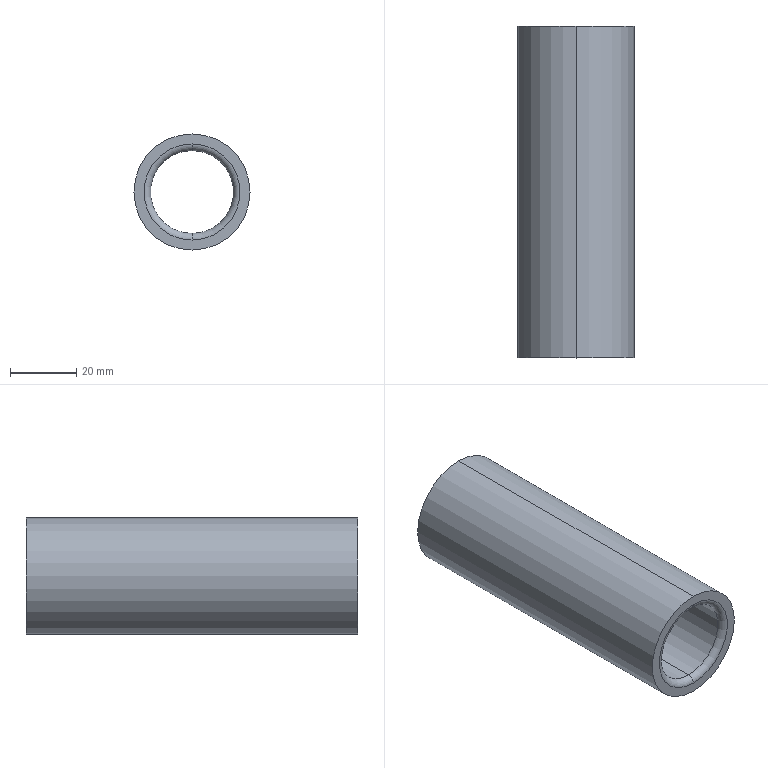Part | SolidWorks | features Extrusion 1, Fillet 1 | 1 solid | 8 faces | box 35 x 100 x 35 mm | volume 47054 mm3 | cylinder 4 | torus 2 | plane 2 | commonest cylinder face diameters 25 x2 35 x2
STEP:
#1=CARTESIAN_POINT('',(0.,2.,-12.5));
#2=VERTEX_POINT('',#1);
#3=CARTESIAN_POINT('',(0.,2.,12.5));
#4=VERTEX_POINT('',#3);
#5=CARTESIAN_POINT('',(0.,2.,0.));
#6=DIRECTION('',(0.,-1.,0.));
#7=DIRECTION('',(0.,0.,1.));
#8=AXIS2_PLACEMENT_3D('',#5,#6,#7);
#9=CIRCLE('',#8,12.5);
#10=EDGE_CURVE('',#2,#4,#9,.T.);
#11=ORIENTED_EDGE('',*,*,#10,.F.);
#12=CARTESIAN_POINT('',(0.,0.,-14.5));
#13=VERTEX_POINT('',#12);
#14=CARTESIAN_POINT('',(0.,2.,-14.5));
#15=DIRECTION('',(1.,0.,0.));
#16=DIRECTION('',(0.,0.,-1.));
#17=AXIS2_PLACEMENT_3D('',#14,#15,#16);
#18=CIRCLE('',#17,2.);
#19=EDGE_CURVE('',#2,#13,#18,.T.);
#20=ORIENTED_EDGE('',*,*,#19,.T.);
#21=CARTESIAN_POINT('',(0.,0.,14.5));
#22=VERTEX_POINT('',#21);
#23=CARTESIAN_POINT('',(0.,0.,0.));
#24=DIRECTION('',(0.,1.,0.));
#25=DIRECTION('',(0.,0.,1.));
#26=AXIS2_PLACEMENT_3D('',#23,#24,#25);
#27=CIRCLE('',#26,14.5);
#28=EDGE_CURVE('',#22,#13,#27,.T.);
#29=ORIENTED_EDGE('',*,*,#28,.F.);
#30=CARTESIAN_POINT('',(0.,2.,14.5));
#31=DIRECTION('',(-1.,0.,0.));
#32=DIRECTION('',(0.,0.,1.));
#33=AXIS2_PLACEMENT_3D('',#30,#31,#32);
#34=CIRCLE('',#33,2.);
#35=EDGE_CURVE('',#4,#22,#34,.T.);
#36=ORIENTED_EDGE('',*,*,#35,.F.);
#37=EDGE_LOOP('',(#11,#20,#29,#36));
#38=FACE_OUTER_BOUND('',#37,.T.);
#39=CARTESIAN_POINT('',(0.,2.,0.));
#40=DIRECTION('',(0.,1.,0.));
#41=DIRECTION('',(0.,0.,1.));
#42=AXIS2_PLACEMENT_3D('',#39,#40,#41);
#43=TOROIDAL_SURFACE('',#42,14.5,2.);
#44=ADVANCED_FACE('',(#38),#43,.T.);
#45=CARTESIAN_POINT('',(0.,100.,-12.5));
#46=VERTEX_POINT('',#45);
#47=CARTESIAN_POINT('',(0.,100.,12.5));
#48=VERTEX_POINT('',#47);
#49=CARTESIAN_POINT('',(0.,100.,0.));
#50=DIRECTION('',(0.,1.,0.));
#51=DIRECTION('',(0.,0.,1.));
#52=AXIS2_PLACEMENT_3D('',#49,#50,#51);
#53=CIRCLE('',#52,12.5);
#54=EDGE_CURVE('',#46,#48,#53,.T.);
#55=ORIENTED_EDGE('',*,*,#54,.T.);
#56=CARTESIAN_POINT('',(0.,100.,12.5));
#57=DIRECTION('',(0.,-1.,0.));
#58=VECTOR('',#57,1000.);
#59=LINE('',#56,#58);
#60=EDGE_CURVE('',#48,#4,#59,.T.);
#61=ORIENTED_EDGE('',*,*,#60,.T.);
#62=CARTESIAN_POINT('',(0.,2.,0.));
#63=DIRECTION('',(0.,-1.,0.));
#64=DIRECTION('',(0.,0.,1.));
#65=AXIS2_PLACEMENT_3D('',#62,#63,#64);
#66=CIRCLE('',#65,12.5);
#67=EDGE_CURVE('',#4,#2,#66,.T.);
#68=ORIENTED_EDGE('',*,*,#67,.T.);
#69=CARTESIAN_POINT('',(0.,100.,-12.5));
#70=DIRECTION('',(0.,-1.,0.));
#71=VECTOR('',#70,1000.);
#72=LINE('',#69,#71);
#73=EDGE_CURVE('',#46,#2,#72,.T.);
#74=ORIENTED_EDGE('',*,*,#73,.F.);
#75=EDGE_LOOP('',(#55,#61,#68,#74));
#76=FACE_OUTER_BOUND('',#75,.T.);
#77=CARTESIAN_POINT('',(0.,100.,0.));
#78=DIRECTION('',(0.,-1.,0.));
#79=DIRECTION('',(0.,0.,-1.));
#80=AXIS2_PLACEMENT_3D('',#77,#78,#79);
#81=CYLINDRICAL_SURFACE('',#80,12.5);
#82=ADVANCED_FACE('',(#76),#81,.F.);
#83=CARTESIAN_POINT('',(0.,100.,17.5));
#84=VERTEX_POINT('',#83);
#85=CARTESIAN_POINT('',(0.,100.,-17.5));
#86=VERTEX_POINT('',#85);
#87=CARTESIAN_POINT('',(0.,100.,0.));
#88=DIRECTION('',(0.,1.,0.));
#89=DIRECTION('',(0.,0.,1.));
#90=AXIS2_PLACEMENT_3D('',#87,#88,#89);
#91=CIRCLE('',#90,17.5);
#92=EDGE_CURVE('',#84,#86,#91,.T.);
#93=ORIENTED_EDGE('',*,*,#92,.F.);
#94=CARTESIAN_POINT('',(0.,0.,17.5));
#95=VERTEX_POINT('',#94);
#96=CARTESIAN_POINT('',(0.,100.,17.5));
#97=DIRECTION('',(0.,-1.,0.));
#98=VECTOR('',#97,1000.);
#99=LINE('',#96,#98);
#100=EDGE_CURVE('',#84,#95,#99,.T.);
#101=ORIENTED_EDGE('',*,*,#100,.T.);
#102=CARTESIAN_POINT('',(0.,0.,-17.5));
#103=VERTEX_POINT('',#102);
#104=CARTESIAN_POINT('',(0.,0.,0.));
#105=DIRECTION('',(0.,1.,0.));
#106=DIRECTION('',(0.,0.,1.));
#107=AXIS2_PLACEMENT_3D('',#104,#105,#106);
#108=CIRCLE('',#107,17.5);
#109=EDGE_CURVE('',#95,#103,#108,.T.);
#110=ORIENTED_EDGE('',*,*,#109,.T.);
#111=CARTESIAN_POINT('',(0.,100.,-17.5));
#112=DIRECTION('',(0.,-1.,0.));
#113=VECTOR('',#112,1000.);
#114=LINE('',#111,#113);
#115=EDGE_CURVE('',#86,#103,#114,.T.);
#116=ORIENTED_EDGE('',*,*,#115,.F.);
#117=EDGE_LOOP('',(#93,#101,#110,#116));
#118=FACE_OUTER_BOUND('',#117,.T.);
#119=CARTESIAN_POINT('',(0.,100.,0.));
#120=DIRECTION('',(0.,-1.,0.));
#121=DIRECTION('',(0.,0.,-1.));
#122=AXIS2_PLACEMENT_3D('',#119,#120,#121);
#123=CYLINDRICAL_SURFACE('',#122,17.5);
#124=ADVANCED_FACE('',(#118),#123,.T.);
#125=CARTESIAN_POINT('',(0.,100.,0.));
#126=DIRECTION('',(0.,1.,0.));
#127=DIRECTION('',(0.,0.,1.));
#128=AXIS2_PLACEMENT_3D('',#125,#126,#127);
#129=CIRCLE('',#128,17.5);
#130=EDGE_CURVE('',#86,#84,#129,.T.);
#131=ORIENTED_EDGE('',*,*,#130,.T.);
#132=ORIENTED_EDGE('',*,*,#92,.T.);
#133=EDGE_LOOP('',(#131,#132));
#134=FACE_OUTER_BOUND('',#133,.T.);
#135=ORIENTED_EDGE('',*,*,#54,.F.);
#136=CARTESIAN_POINT('',(0.,100.,0.));
#137=DIRECTION('',(0.,1.,0.));
#138=DIRECTION('',(0.,0.,1.));
#139=AXIS2_PLACEMENT_3D('',#136,#137,#138);
#140=CIRCLE('',#139,12.5);
#141=EDGE_CURVE('',#48,#46,#140,.T.);
#142=ORIENTED_EDGE('',*,*,#141,.F.);
#143=EDGE_LOOP('',(#135,#142));
#144=FACE_BOUND('',#143,.T.);
#145=CARTESIAN_POINT('',(0.,100.,0.));
#146=DIRECTION('',(0.,1.,0.));
#147=DIRECTION('',(0.,0.,1.));
#148=AXIS2_PLACEMENT_3D('',#145,#146,#147);
#149=PLANE('',#148);
#150=ADVANCED_FACE('',(#134,#144),#149,.T.);
#151=ORIENTED_EDGE('',*,*,#28,.T.);
#152=CARTESIAN_POINT('',(0.,0.,0.));
#153=DIRECTION('',(0.,1.,0.));
#154=DIRECTION('',(0.,0.,1.));
#155=AXIS2_PLACEMENT_3D('',#152,#153,#154);
#156=CIRCLE('',#155,14.5);
#157=EDGE_CURVE('',#13,#22,#156,.T.);
#158=ORIENTED_EDGE('',*,*,#157,.T.);
#159=EDGE_LOOP('',(#151,#158));
#160=FACE_BOUND('',#159,.T.);
#161=CARTESIAN_POINT('',(0.,0.,0.));
#162=DIRECTION('',(0.,1.,0.));
#163=DIRECTION('',(0.,0.,1.));
#164=AXIS2_PLACEMENT_3D('',#161,#162,#163);
#165=CIRCLE('',#164,17.5);
#166=EDGE_CURVE('',#103,#95,#165,.T.);
#167=ORIENTED_EDGE('',*,*,#166,.F.);
#168=ORIENTED_EDGE('',*,*,#109,.F.);
#169=EDGE_LOOP('',(#167,#168));
#170=FACE_OUTER_BOUND('',#169,.T.);
#171=CARTESIAN_POINT('',(0.,0.,0.));
#172=DIRECTION('',(0.,1.,0.));
#173=DIRECTION('',(0.,0.,1.));
#174=AXIS2_PLACEMENT_3D('',#171,#172,#173);
#175=PLANE('',#174);
#176=ADVANCED_FACE('',(#160,#170),#175,.F.);
#177=ORIENTED_EDGE('',*,*,#100,.F.);
#178=ORIENTED_EDGE('',*,*,#130,.F.);
#179=ORIENTED_EDGE('',*,*,#115,.T.);
#180=ORIENTED_EDGE('',*,*,#166,.T.);
#181=EDGE_LOOP('',(#177,#178,#179,#180));
#182=FACE_OUTER_BOUND('',#181,.T.);
#183=CARTESIAN_POINT('',(0.,100.,0.));
#184=DIRECTION('',(0.,-1.,0.));
#185=DIRECTION('',(0.,0.,-1.));
#186=AXIS2_PLACEMENT_3D('',#183,#184,#185);
#187=CYLINDRICAL_SURFACE('',#186,17.5);
#188=ADVANCED_FACE('',(#182),#187,.T.);
#189=ORIENTED_EDGE('',*,*,#60,.F.);
#190=ORIENTED_EDGE('',*,*,#141,.T.);
#191=ORIENTED_EDGE('',*,*,#73,.T.);
#192=ORIENTED_EDGE('',*,*,#10,.T.);
#193=EDGE_LOOP('',(#189,#190,#191,#192));
#194=FACE_OUTER_BOUND('',#193,.T.);
#195=CARTESIAN_POINT('',(0.,100.,0.));
#196=DIRECTION('',(0.,-1.,0.));
#197=DIRECTION('',(0.,0.,-1.));
#198=AXIS2_PLACEMENT_3D('',#195,#196,#197);
#199=CYLINDRICAL_SURFACE('',#198,12.5);
#200=ADVANCED_FACE('',(#194),#199,.F.);
#201=ORIENTED_EDGE('',*,*,#19,.F.);
#202=ORIENTED_EDGE('',*,*,#67,.F.);
#203=ORIENTED_EDGE('',*,*,#35,.T.);
#204=ORIENTED_EDGE('',*,*,#157,.F.);
#205=EDGE_LOOP('',(#201,#202,#203,#204));
#206=FACE_OUTER_BOUND('',#205,.T.);
#207=CARTESIAN_POINT('',(0.,2.,0.));
#208=DIRECTION('',(0.,1.,0.));
#209=DIRECTION('',(0.,0.,1.));
#210=AXIS2_PLACEMENT_3D('',#207,#208,#209);
#211=TOROIDAL_SURFACE('',#210,14.5,2.);
#212=ADVANCED_FACE('',(#206),#211,.T.);
#213=CLOSED_SHELL('',(#44,#82,#124,#150,#176,#188,#200,#212));
#214=MANIFOLD_SOLID_BREP('',#213);
#215=CARTESIAN_POINT('',(0.,0.,0.));
#216=DIRECTION('',(0.,0.,1.));
#217=DIRECTION('',(1.,0.,0.));
#218=AXIS2_PLACEMENT_3D('',#215,#216,#217);
#219=(LENGTH_UNIT()NAMED_UNIT(*)SI_UNIT(.MILLI.,.METRE.));
#220=UNCERTAINTY_MEASURE_WITH_UNIT(LENGTH_MEASURE(0.00001),#219,'','');
#221=(NAMED_UNIT(*)PLANE_ANGLE_UNIT()SI_UNIT($,.RADIAN.));
#222=(NAMED_UNIT(*)SI_UNIT($,.STERADIAN.)SOLID_ANGLE_UNIT());
#223=(GEOMETRIC_REPRESENTATION_CONTEXT(3)GLOBAL_UNCERTAINTY_ASSIGNED_CONTEXT((#220))GLOBAL_UNIT_ASSIGNED_CONTEXT((#219,#221,#222))REPRESENTATION_CONTEXT('',''));
#224=ADVANCED_BREP_SHAPE_REPRESENTATION('',(#214,#218),#223);